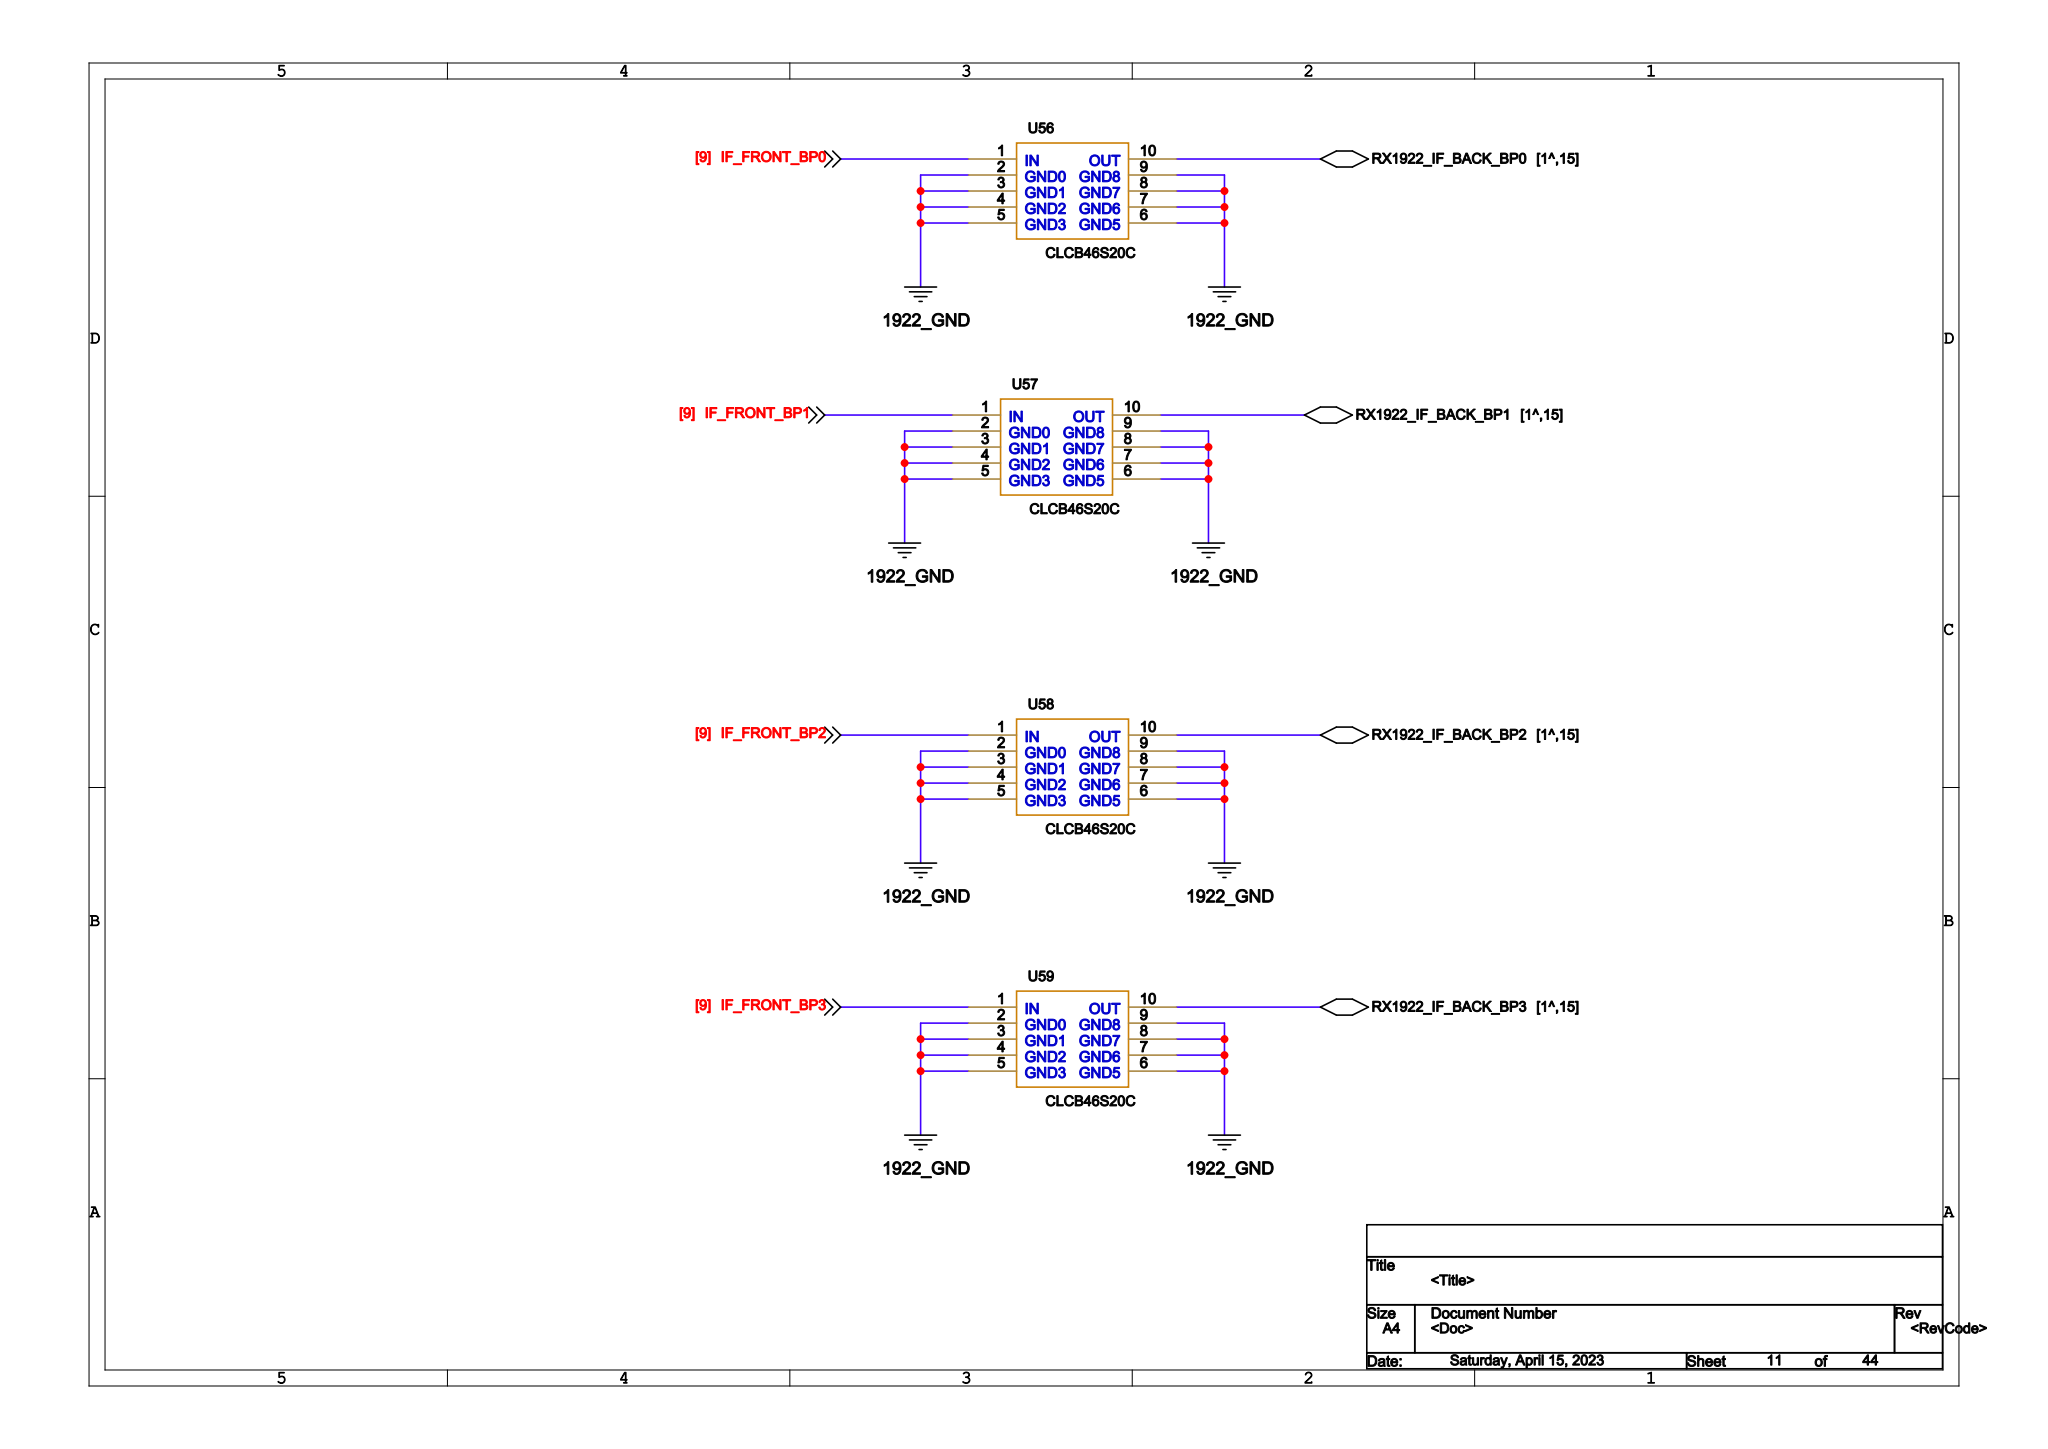Circuit board | Cadence Allegro | 1034 parts | 912 nets | one sheet of the schematic
Parts on this sheet (reference | value | footprint):
U56 | CLCB46S20C | CLCB46S20C
U57 | CLCB46S20C | CLCB46S20C
U58 | CLCB46S20C | CLCB46S20C
U59 | CLCB46S20C | CLCB46S20C
Nets of these parts (net: part-pin ...):
IF_FRONT_BP0_D2: U56-1
IF_FRONT_BP1_D2: U57-1
IF_FRONT_BP2_D2: U58-1
IF_FRONT_BP3_D2: U59-1
1922_GND: U56-2 U56-3 U56-4 U56-5 U56-6 U56-7 U56-8 U56-9 U57-2 U57-3 U57-4 U57-5 U57-6 U57-7 U57-8 U57-9 U58-2 U58-3 U58-4 U58-5 U58-6 U58-7 U58-8 U58-9 U59-2 U59-3 U59-4 U59-5 U59-6 U59-7 U59-8 U59-9
N186408: U57-10
N186410: U58-10
N186406: U56-10
N186412: U59-10